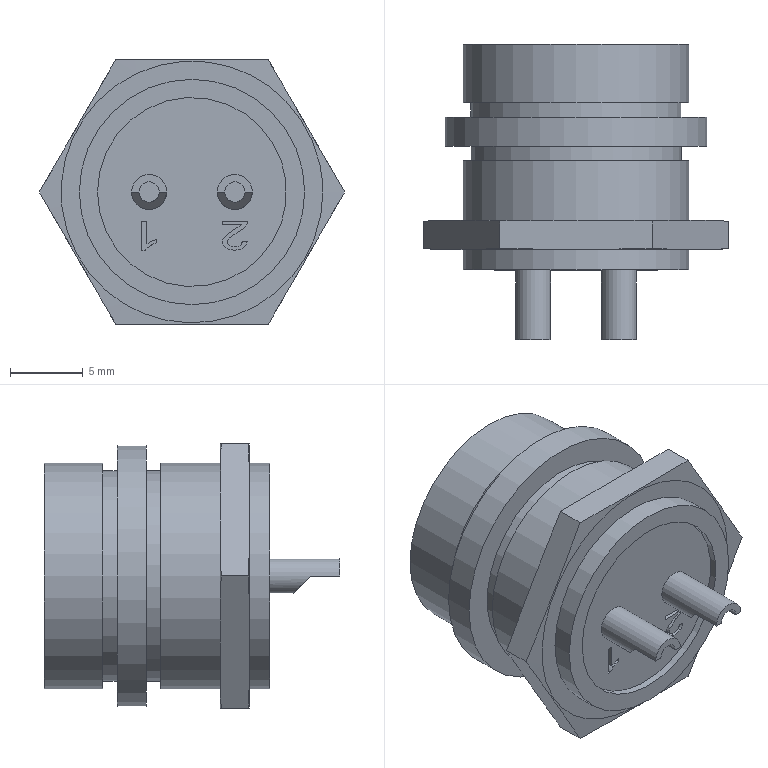Part | STEP file | EN80200001 | 2 solids | 83 faces | box 21 x 20.3 x 18.187 mm | volume 1904 mm3 | plane 44 | other 18 | cylinder 15 | sphere 4 | spline 2 | commonest cylinder face diameters 2.4 x4 15.5 x3 1.4 x2 13 x2 14.5 x2 2 x1